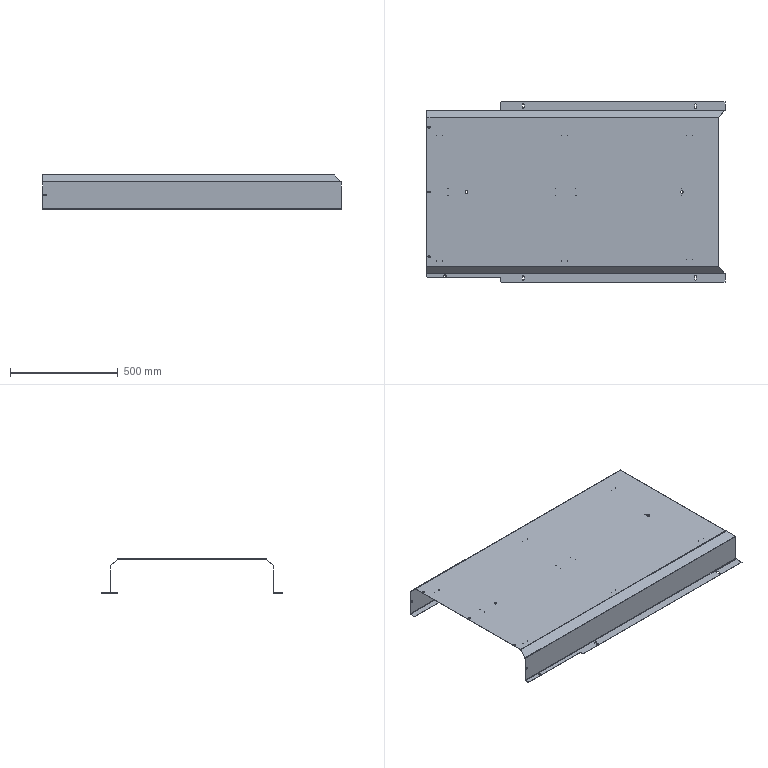Part | NX | features solid 2 | 1 solid | 137 faces | box 1383 x 836 x 160 mm | volume 1807429 mm3 | cylinder 86 | plane 47 | spline 4 | commonest cylinder face diameters 1 x40 7 x13 9 x8 2.4 x7 4.8 x7 10 x5